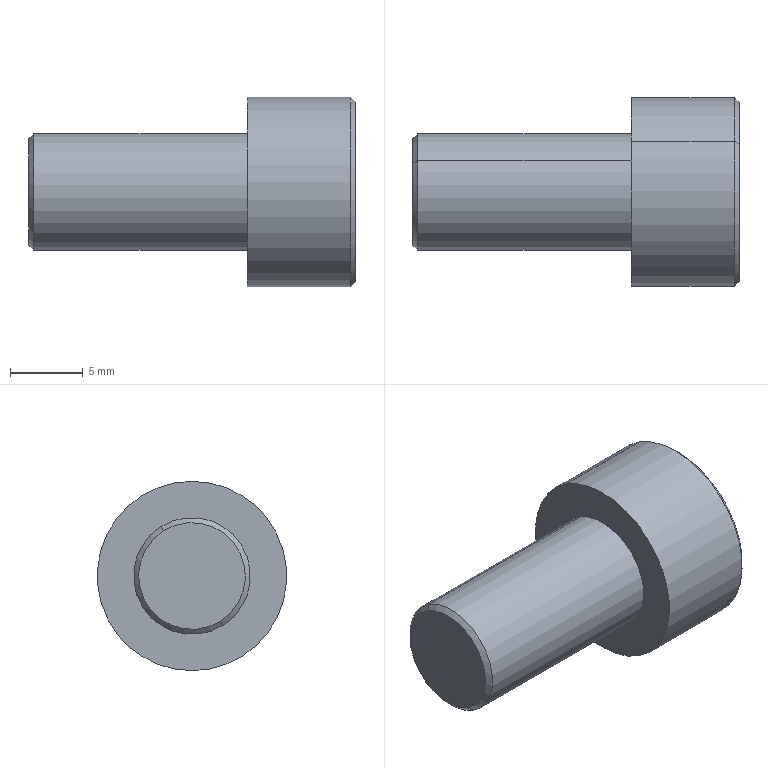Part | STEP file | M8_NL23(L=15) | 1 solid | 18 faces | box 22.4 x 12.98 x 12.98 mm | volume 1605 mm3 | plane 10 | cylinder 4 | cone 4 | commonest cylinder face diameters 8 x2 12.98 x2